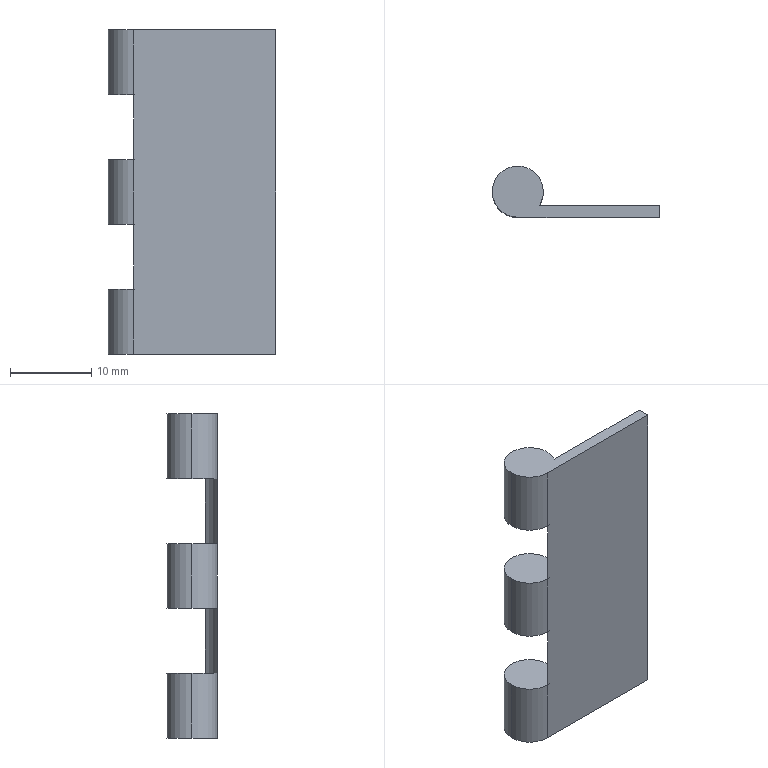Part | SolidWorks | features BaseBody 1 | 1 solid | 20 faces | box 20.65 x 6.3 x 40 mm | volume 1684 mm3 | cylinder 11 | plane 9 | commonest cylinder face diameters 6.3 x11
STEP:
#1=CARTESIAN_POINT('',(3.15,3.15,32.));
#2=VERTEX_POINT('',#1);
#3=CARTESIAN_POINT('',(-3.15,3.15,32.));
#4=VERTEX_POINT('',#3);
#5=CARTESIAN_POINT('',(0.,3.15,32.));
#6=DIRECTION('',(0.,0.,1.));
#7=DIRECTION('',(1.,0.,0.));
#8=AXIS2_PLACEMENT_3D('',#5,#6,#7);
#9=CIRCLE('',#8,3.15);
#10=EDGE_CURVE('',#2,#4,#9,.T.);
#11=ORIENTED_EDGE('',*,*,#10,.T.);
#12=CARTESIAN_POINT('',(-3.15,3.15,40.));
#13=VERTEX_POINT('',#12);
#14=CARTESIAN_POINT('',(-3.15,3.15,40.));
#15=DIRECTION('',(0.,0.,1.));
#16=VECTOR('',#15,1000.);
#17=LINE('',#14,#16);
#18=EDGE_CURVE('',#4,#13,#17,.T.);
#19=ORIENTED_EDGE('',*,*,#18,.T.);
#20=CARTESIAN_POINT('',(3.15,3.15,40.));
#21=VERTEX_POINT('',#20);
#22=CARTESIAN_POINT('',(0.,3.15,40.));
#23=DIRECTION('',(0.,0.,1.));
#24=DIRECTION('',(1.,0.,0.));
#25=AXIS2_PLACEMENT_3D('',#22,#23,#24);
#26=CIRCLE('',#25,3.15);
#27=EDGE_CURVE('',#21,#13,#26,.T.);
#28=ORIENTED_EDGE('',*,*,#27,.F.);
#29=CARTESIAN_POINT('',(3.15,3.15,40.));
#30=DIRECTION('',(0.,0.,1.));
#31=VECTOR('',#30,1000.);
#32=LINE('',#29,#31);
#33=EDGE_CURVE('',#2,#21,#32,.T.);
#34=ORIENTED_EDGE('',*,*,#33,.F.);
#35=EDGE_LOOP('',(#11,#19,#28,#34));
#36=FACE_OUTER_BOUND('',#35,.T.);
#37=CARTESIAN_POINT('',(0.,3.15,40.));
#38=DIRECTION('',(0.,0.,1.));
#39=DIRECTION('',(1.,0.,0.));
#40=AXIS2_PLACEMENT_3D('',#37,#38,#39);
#41=CYLINDRICAL_SURFACE('',#40,3.15);
#42=ADVANCED_FACE('',(#36),#41,.T.);
#43=CARTESIAN_POINT('',(2.683,1.5,32.));
#44=VERTEX_POINT('',#43);
#45=CARTESIAN_POINT('',(0.,3.15,32.));
#46=DIRECTION('',(0.,0.,1.));
#47=DIRECTION('',(1.,0.,0.));
#48=AXIS2_PLACEMENT_3D('',#45,#46,#47);
#49=CIRCLE('',#48,3.15);
#50=EDGE_CURVE('',#44,#2,#49,.T.);
#51=ORIENTED_EDGE('',*,*,#50,.T.);
#52=ORIENTED_EDGE('',*,*,#33,.T.);
#53=CARTESIAN_POINT('',(2.683,1.5,40.));
#54=VERTEX_POINT('',#53);
#55=CARTESIAN_POINT('',(0.,3.15,40.));
#56=DIRECTION('',(0.,0.,1.));
#57=DIRECTION('',(1.,0.,0.));
#58=AXIS2_PLACEMENT_3D('',#55,#56,#57);
#59=CIRCLE('',#58,3.15);
#60=EDGE_CURVE('',#54,#21,#59,.T.);
#61=ORIENTED_EDGE('',*,*,#60,.F.);
#62=CARTESIAN_POINT('',(2.683,1.5,40.));
#63=DIRECTION('',(0.,0.,-1.));
#64=VECTOR('',#63,1000.);
#65=LINE('',#62,#64);
#66=EDGE_CURVE('',#54,#44,#65,.T.);
#67=ORIENTED_EDGE('',*,*,#66,.T.);
#68=EDGE_LOOP('',(#51,#52,#61,#67));
#69=FACE_OUTER_BOUND('',#68,.T.);
#70=CARTESIAN_POINT('',(0.,3.15,40.));
#71=DIRECTION('',(0.,0.,1.));
#72=DIRECTION('',(1.,0.,0.));
#73=AXIS2_PLACEMENT_3D('',#70,#71,#72);
#74=CYLINDRICAL_SURFACE('',#73,3.15);
#75=ADVANCED_FACE('',(#69),#74,.T.);
#76=CARTESIAN_POINT('',(3.15,3.15,16.));
#77=VERTEX_POINT('',#76);
#78=CARTESIAN_POINT('',(-3.15,3.15,16.));
#79=VERTEX_POINT('',#78);
#80=CARTESIAN_POINT('',(0.,3.15,16.));
#81=DIRECTION('',(0.,0.,1.));
#82=DIRECTION('',(1.,0.,0.));
#83=AXIS2_PLACEMENT_3D('',#80,#81,#82);
#84=CIRCLE('',#83,3.15);
#85=EDGE_CURVE('',#77,#79,#84,.T.);
#86=ORIENTED_EDGE('',*,*,#85,.T.);
#87=CARTESIAN_POINT('',(-3.15,3.15,24.));
#88=VERTEX_POINT('',#87);
#89=CARTESIAN_POINT('',(-3.15,3.15,40.));
#90=DIRECTION('',(0.,0.,1.));
#91=VECTOR('',#90,1000.);
#92=LINE('',#89,#91);
#93=EDGE_CURVE('',#79,#88,#92,.T.);
#94=ORIENTED_EDGE('',*,*,#93,.T.);
#95=CARTESIAN_POINT('',(3.15,3.15,24.));
#96=VERTEX_POINT('',#95);
#97=CARTESIAN_POINT('',(0.,3.15,24.));
#98=DIRECTION('',(0.,0.,-1.));
#99=DIRECTION('',(1.,0.,0.));
#100=AXIS2_PLACEMENT_3D('',#97,#98,#99);
#101=CIRCLE('',#100,3.15);
#102=EDGE_CURVE('',#88,#96,#101,.T.);
#103=ORIENTED_EDGE('',*,*,#102,.T.);
#104=CARTESIAN_POINT('',(3.15,3.15,40.));
#105=DIRECTION('',(0.,0.,1.));
#106=VECTOR('',#105,1000.);
#107=LINE('',#104,#106);
#108=EDGE_CURVE('',#77,#96,#107,.T.);
#109=ORIENTED_EDGE('',*,*,#108,.F.);
#110=EDGE_LOOP('',(#86,#94,#103,#109));
#111=FACE_OUTER_BOUND('',#110,.T.);
#112=CARTESIAN_POINT('',(0.,3.15,40.));
#113=DIRECTION('',(0.,0.,1.));
#114=DIRECTION('',(1.,0.,0.));
#115=AXIS2_PLACEMENT_3D('',#112,#113,#114);
#116=CYLINDRICAL_SURFACE('',#115,3.15);
#117=ADVANCED_FACE('',(#111),#116,.T.);
#118=CARTESIAN_POINT('',(2.683,1.5,16.));
#119=VERTEX_POINT('',#118);
#120=CARTESIAN_POINT('',(0.,3.15,16.));
#121=DIRECTION('',(0.,0.,1.));
#122=DIRECTION('',(1.,0.,0.));
#123=AXIS2_PLACEMENT_3D('',#120,#121,#122);
#124=CIRCLE('',#123,3.15);
#125=EDGE_CURVE('',#119,#77,#124,.T.);
#126=ORIENTED_EDGE('',*,*,#125,.T.);
#127=ORIENTED_EDGE('',*,*,#108,.T.);
#128=CARTESIAN_POINT('',(2.683,1.5,24.));
#129=VERTEX_POINT('',#128);
#130=CARTESIAN_POINT('',(0.,3.15,24.));
#131=DIRECTION('',(0.,0.,-1.));
#132=DIRECTION('',(1.,0.,0.));
#133=AXIS2_PLACEMENT_3D('',#130,#131,#132);
#134=CIRCLE('',#133,3.15);
#135=EDGE_CURVE('',#96,#129,#134,.T.);
#136=ORIENTED_EDGE('',*,*,#135,.T.);
#137=CARTESIAN_POINT('',(2.683,1.5,40.));
#138=DIRECTION('',(0.,0.,-1.));
#139=VECTOR('',#138,1000.);
#140=LINE('',#137,#139);
#141=EDGE_CURVE('',#129,#119,#140,.T.);
#142=ORIENTED_EDGE('',*,*,#141,.T.);
#143=EDGE_LOOP('',(#126,#127,#136,#142));
#144=FACE_OUTER_BOUND('',#143,.T.);
#145=CARTESIAN_POINT('',(0.,3.15,40.));
#146=DIRECTION('',(0.,0.,1.));
#147=DIRECTION('',(1.,0.,0.));
#148=AXIS2_PLACEMENT_3D('',#145,#146,#147);
#149=CYLINDRICAL_SURFACE('',#148,3.15);
#150=ADVANCED_FACE('',(#144),#149,.T.);
#151=CARTESIAN_POINT('',(3.15,3.15,0.));
#152=VERTEX_POINT('',#151);
#153=CARTESIAN_POINT('',(-3.15,3.15,0.));
#154=VERTEX_POINT('',#153);
#155=CARTESIAN_POINT('',(0.,3.15,0.));
#156=DIRECTION('',(0.,0.,1.));
#157=DIRECTION('',(1.,0.,0.));
#158=AXIS2_PLACEMENT_3D('',#155,#156,#157);
#159=CIRCLE('',#158,3.15);
#160=EDGE_CURVE('',#152,#154,#159,.T.);
#161=ORIENTED_EDGE('',*,*,#160,.T.);
#162=CARTESIAN_POINT('',(-3.15,3.15,8.));
#163=VERTEX_POINT('',#162);
#164=CARTESIAN_POINT('',(-3.15,3.15,40.));
#165=DIRECTION('',(0.,0.,1.));
#166=VECTOR('',#165,1000.);
#167=LINE('',#164,#166);
#168=EDGE_CURVE('',#154,#163,#167,.T.);
#169=ORIENTED_EDGE('',*,*,#168,.T.);
#170=CARTESIAN_POINT('',(3.15,3.15,8.));
#171=VERTEX_POINT('',#170);
#172=CARTESIAN_POINT('',(0.,3.15,8.));
#173=DIRECTION('',(0.,0.,-1.));
#174=DIRECTION('',(1.,0.,0.));
#175=AXIS2_PLACEMENT_3D('',#172,#173,#174);
#176=CIRCLE('',#175,3.15);
#177=EDGE_CURVE('',#163,#171,#176,.T.);
#178=ORIENTED_EDGE('',*,*,#177,.T.);
#179=CARTESIAN_POINT('',(3.15,3.15,40.));
#180=DIRECTION('',(0.,0.,1.));
#181=VECTOR('',#180,1000.);
#182=LINE('',#179,#181);
#183=EDGE_CURVE('',#152,#171,#182,.T.);
#184=ORIENTED_EDGE('',*,*,#183,.F.);
#185=EDGE_LOOP('',(#161,#169,#178,#184));
#186=FACE_OUTER_BOUND('',#185,.T.);
#187=CARTESIAN_POINT('',(0.,3.15,40.));
#188=DIRECTION('',(0.,0.,1.));
#189=DIRECTION('',(1.,0.,0.));
#190=AXIS2_PLACEMENT_3D('',#187,#188,#189);
#191=CYLINDRICAL_SURFACE('',#190,3.15);
#192=ADVANCED_FACE('',(#186),#191,.T.);
#193=CARTESIAN_POINT('',(2.683,1.5,0.));
#194=VERTEX_POINT('',#193);
#195=CARTESIAN_POINT('',(0.,3.15,0.));
#196=DIRECTION('',(0.,0.,1.));
#197=DIRECTION('',(1.,0.,0.));
#198=AXIS2_PLACEMENT_3D('',#195,#196,#197);
#199=CIRCLE('',#198,3.15);
#200=EDGE_CURVE('',#194,#152,#199,.T.);
#201=ORIENTED_EDGE('',*,*,#200,.T.);
#202=ORIENTED_EDGE('',*,*,#183,.T.);
#203=CARTESIAN_POINT('',(2.683,1.5,8.));
#204=VERTEX_POINT('',#203);
#205=CARTESIAN_POINT('',(0.,3.15,8.));
#206=DIRECTION('',(0.,0.,-1.));
#207=DIRECTION('',(1.,0.,0.));
#208=AXIS2_PLACEMENT_3D('',#205,#206,#207);
#209=CIRCLE('',#208,3.15);
#210=EDGE_CURVE('',#171,#204,#209,.T.);
#211=ORIENTED_EDGE('',*,*,#210,.T.);
#212=CARTESIAN_POINT('',(2.683,1.5,40.));
#213=DIRECTION('',(0.,0.,-1.));
#214=VECTOR('',#213,1000.);
#215=LINE('',#212,#214);
#216=EDGE_CURVE('',#204,#194,#215,.T.);
#217=ORIENTED_EDGE('',*,*,#216,.T.);
#218=EDGE_LOOP('',(#201,#202,#211,#217));
#219=FACE_OUTER_BOUND('',#218,.T.);
#220=CARTESIAN_POINT('',(0.,3.15,40.));
#221=DIRECTION('',(0.,0.,1.));
#222=DIRECTION('',(1.,0.,0.));
#223=AXIS2_PLACEMENT_3D('',#220,#221,#222);
#224=CYLINDRICAL_SURFACE('',#223,3.15);
#225=ADVANCED_FACE('',(#219),#224,.T.);
#226=CARTESIAN_POINT('',(17.5,0.,40.));
#227=VERTEX_POINT('',#226);
#228=CARTESIAN_POINT('',(17.5,0.,0.));
#229=VERTEX_POINT('',#228);
#230=CARTESIAN_POINT('',(17.5,0.,40.));
#231=DIRECTION('',(0.,0.,-1.));
#232=VECTOR('',#231,1000.);
#233=LINE('',#230,#232);
#234=EDGE_CURVE('',#227,#229,#233,.T.);
#235=ORIENTED_EDGE('',*,*,#234,.F.);
#236=CARTESIAN_POINT('',(0.,0.,40.));
#237=VERTEX_POINT('',#236);
#238=CARTESIAN_POINT('',(0.,0.,40.));
#239=DIRECTION('',(1.,0.,0.));
#240=VECTOR('',#239,1000.);
#241=LINE('',#238,#240);
#242=EDGE_CURVE('',#237,#227,#241,.T.);
#243=ORIENTED_EDGE('',*,*,#242,.F.);
#244=CARTESIAN_POINT('',(0.,0.,32.));
#245=VERTEX_POINT('',#244);
#246=CARTESIAN_POINT('',(0.,0.,40.));
#247=DIRECTION('',(0.,0.,1.));
#248=VECTOR('',#247,1000.);
#249=LINE('',#246,#248);
#250=EDGE_CURVE('',#245,#237,#249,.T.);
#251=ORIENTED_EDGE('',*,*,#250,.F.);
#252=CARTESIAN_POINT('',(0.,0.,24.));
#253=VERTEX_POINT('',#252);
#254=CARTESIAN_POINT('',(0.,0.,40.));
#255=DIRECTION('',(0.,0.,1.));
#256=VECTOR('',#255,1000.);
#257=LINE('',#254,#256);
#258=EDGE_CURVE('',#253,#245,#257,.T.);
#259=ORIENTED_EDGE('',*,*,#258,.F.);
#260=CARTESIAN_POINT('',(0.,0.,16.));
#261=VERTEX_POINT('',#260);
#262=CARTESIAN_POINT('',(0.,0.,40.));
#263=DIRECTION('',(0.,0.,1.));
#264=VECTOR('',#263,1000.);
#265=LINE('',#262,#264);
#266=EDGE_CURVE('',#261,#253,#265,.T.);
#267=ORIENTED_EDGE('',*,*,#266,.F.);
#268=CARTESIAN_POINT('',(0.,0.,8.));
#269=VERTEX_POINT('',#268);
#270=CARTESIAN_POINT('',(0.,0.,40.));
#271=DIRECTION('',(0.,0.,1.));
#272=VECTOR('',#271,1000.);
#273=LINE('',#270,#272);
#274=EDGE_CURVE('',#269,#261,#273,.T.);
#275=ORIENTED_EDGE('',*,*,#274,.F.);
#276=CARTESIAN_POINT('',(0.,0.,0.));
#277=VERTEX_POINT('',#276);
#278=CARTESIAN_POINT('',(0.,0.,40.));
#279=DIRECTION('',(0.,0.,1.));
#280=VECTOR('',#279,1000.);
#281=LINE('',#278,#280);
#282=EDGE_CURVE('',#277,#269,#281,.T.);
#283=ORIENTED_EDGE('',*,*,#282,.F.);
#284=CARTESIAN_POINT('',(0.,0.,0.));
#285=DIRECTION('',(-1.,0.,0.));
#286=VECTOR('',#285,1000.);
#287=LINE('',#284,#286);
#288=EDGE_CURVE('',#229,#277,#287,.T.);
#289=ORIENTED_EDGE('',*,*,#288,.F.);
#290=EDGE_LOOP('',(#235,#243,#251,#259,#267,#275,#283,#289));
#291=FACE_OUTER_BOUND('',#290,.T.);
#292=CARTESIAN_POINT('',(0.,0.,40.));
#293=DIRECTION('',(0.,1.,0.));
#294=DIRECTION('',(0.,0.,1.));
#295=AXIS2_PLACEMENT_3D('',#292,#293,#294);
#296=PLANE('',#295);
#297=ADVANCED_FACE('',(#291),#296,.F.);
#298=CARTESIAN_POINT('',(17.5,1.5,0.));
#299=VERTEX_POINT('',#298);
#300=CARTESIAN_POINT('',(17.5,3.15,0.));
#301=DIRECTION('',(0.,1.,0.));
#302=VECTOR('',#301,1000.);
#303=LINE('',#300,#302);
#304=EDGE_CURVE('',#229,#299,#303,.T.);
#305=ORIENTED_EDGE('',*,*,#304,.F.);
#306=ORIENTED_EDGE('',*,*,#288,.T.);
#307=CARTESIAN_POINT('',(0.,3.15,0.));
#308=DIRECTION('',(0.,0.,1.));
#309=DIRECTION('',(1.,0.,0.));
#310=AXIS2_PLACEMENT_3D('',#307,#308,#309);
#311=CIRCLE('',#310,3.15);
#312=EDGE_CURVE('',#154,#277,#311,.T.);
#313=ORIENTED_EDGE('',*,*,#312,.F.);
#314=ORIENTED_EDGE('',*,*,#160,.F.);
#315=ORIENTED_EDGE('',*,*,#200,.F.);
#316=CARTESIAN_POINT('',(0.,1.5,0.));
#317=DIRECTION('',(-1.,0.,0.));
#318=VECTOR('',#317,1000.);
#319=LINE('',#316,#318);
#320=EDGE_CURVE('',#299,#194,#319,.T.);
#321=ORIENTED_EDGE('',*,*,#320,.F.);
#322=EDGE_LOOP('',(#305,#306,#313,#314,#315,#321));
#323=FACE_OUTER_BOUND('',#322,.T.);
#324=CARTESIAN_POINT('',(0.,3.15,0.));
#325=DIRECTION('',(0.,0.,1.));
#326=DIRECTION('',(1.,0.,0.));
#327=AXIS2_PLACEMENT_3D('',#324,#325,#326);
#328=PLANE('',#327);
#329=ADVANCED_FACE('',(#323),#328,.F.);
#330=CARTESIAN_POINT('',(17.5,1.5,40.));
#331=VERTEX_POINT('',#330);
#332=CARTESIAN_POINT('',(17.5,1.5,40.));
#333=DIRECTION('',(0.,0.,-1.));
#334=VECTOR('',#333,1000.);
#335=LINE('',#332,#334);
#336=EDGE_CURVE('',#331,#299,#335,.T.);
#337=ORIENTED_EDGE('',*,*,#336,.F.);
#338=CARTESIAN_POINT('',(17.5,0.,40.));
#339=DIRECTION('',(0.,1.,0.));
#340=VECTOR('',#339,1000.);
#341=LINE('',#338,#340);
#342=EDGE_CURVE('',#227,#331,#341,.T.);
#343=ORIENTED_EDGE('',*,*,#342,.F.);
#344=ORIENTED_EDGE('',*,*,#234,.T.);
#345=ORIENTED_EDGE('',*,*,#304,.T.);
#346=EDGE_LOOP('',(#337,#343,#344,#345));
#347=FACE_OUTER_BOUND('',#346,.T.);
#348=CARTESIAN_POINT('',(17.5,0.,40.));
#349=DIRECTION('',(-1.,0.,0.));
#350=DIRECTION('',(0.,0.,1.));
#351=AXIS2_PLACEMENT_3D('',#348,#349,#350);
#352=PLANE('',#351);
#353=ADVANCED_FACE('',(#347),#352,.F.);
#354=ORIENTED_EDGE('',*,*,#242,.T.);
#355=ORIENTED_EDGE('',*,*,#342,.T.);
#356=CARTESIAN_POINT('',(0.,1.5,40.));
#357=DIRECTION('',(-1.,0.,0.));
#358=VECTOR('',#357,1000.);
#359=LINE('',#356,#358);
#360=EDGE_CURVE('',#331,#54,#359,.T.);
#361=ORIENTED_EDGE('',*,*,#360,.T.);
#362=ORIENTED_EDGE('',*,*,#60,.T.);
#363=ORIENTED_EDGE('',*,*,#27,.T.);
#364=CARTESIAN_POINT('',(0.,3.15,40.));
#365=DIRECTION('',(0.,0.,1.));
#366=DIRECTION('',(1.,0.,0.));
#367=AXIS2_PLACEMENT_3D('',#364,#365,#366);
#368=CIRCLE('',#367,3.15);
#369=EDGE_CURVE('',#13,#237,#368,.T.);
#370=ORIENTED_EDGE('',*,*,#369,.T.);
#371=EDGE_LOOP('',(#354,#355,#361,#362,#363,#370));
#372=FACE_OUTER_BOUND('',#371,.T.);
#373=CARTESIAN_POINT('',(0.,3.15,40.));
#374=DIRECTION('',(0.,0.,1.));
#375=DIRECTION('',(1.,0.,0.));
#376=AXIS2_PLACEMENT_3D('',#373,#374,#375);
#377=PLANE('',#376);
#378=ADVANCED_FACE('',(#372),#377,.T.);
#379=ORIENTED_EDGE('',*,*,#18,.F.);
#380=CARTESIAN_POINT('',(0.,3.15,32.));
#381=DIRECTION('',(0.,0.,1.));
#382=DIRECTION('',(1.,0.,0.));
#383=AXIS2_PLACEMENT_3D('',#380,#381,#382);
#384=CIRCLE('',#383,3.15);
#385=EDGE_CURVE('',#4,#245,#384,.T.);
#386=ORIENTED_EDGE('',*,*,#385,.T.);
#387=ORIENTED_EDGE('',*,*,#250,.T.);
#388=ORIENTED_EDGE('',*,*,#369,.F.);
#389=EDGE_LOOP('',(#379,#386,#387,#388));
#390=FACE_OUTER_BOUND('',#389,.T.);
#391=CARTESIAN_POINT('',(0.,3.15,40.));
#392=DIRECTION('',(0.,0.,1.));
#393=DIRECTION('',(1.,0.,0.));
#394=AXIS2_PLACEMENT_3D('',#391,#392,#393);
#395=CYLINDRICAL_SURFACE('',#394,3.15);
#396=ADVANCED_FACE('',(#390),#395,.T.);
#397=CARTESIAN_POINT('',(0.,3.15,24.));
#398=DIRECTION('',(0.,0.,1.));
#399=DIRECTION('',(1.,0.,0.));
#400=AXIS2_PLACEMENT_3D('',#397,#398,#399);
#401=CIRCLE('',#400,3.15);
#402=EDGE_CURVE('',#253,#129,#401,.T.);
#403=ORIENTED_EDGE('',*,*,#402,.F.);
#404=ORIENTED_EDGE('',*,*,#258,.T.);
#405=CARTESIAN_POINT('',(0.,3.15,32.));
#406=DIRECTION('',(0.,0.,-1.));
#407=DIRECTION('',(1.,0.,0.));
#408=AXIS2_PLACEMENT_3D('',#405,#406,#407);
#409=CIRCLE('',#408,3.15);
#410=EDGE_CURVE('',#44,#245,#409,.T.);
#411=ORIENTED_EDGE('',*,*,#410,.F.);
#412=CARTESIAN_POINT('',(2.683,1.5,32.));
#413=DIRECTION('',(0.,0.,1.));
#414=VECTOR('',#413,1000.);
#415=LINE('',#412,#414);
#416=EDGE_CURVE('',#129,#44,#415,.T.);
#417=ORIENTED_EDGE('',*,*,#416,.F.);
#418=EDGE_LOOP('',(#403,#404,#411,#417));
#419=FACE_OUTER_BOUND('',#418,.T.);
#420=CARTESIAN_POINT('',(0.,3.15,32.));
#421=DIRECTION('',(0.,0.,1.));
#422=DIRECTION('',(1.,0.,0.));
#423=AXIS2_PLACEMENT_3D('',#420,#421,#422);
#424=CYLINDRICAL_SURFACE('',#423,3.15);
#425=ADVANCED_FACE('',(#419),#424,.F.);
#426=ORIENTED_EDGE('',*,*,#93,.F.);
#427=CARTESIAN_POINT('',(0.,3.15,16.));
#428=DIRECTION('',(0.,0.,1.));
#429=DIRECTION('',(1.,0.,0.));
#430=AXIS2_PLACEMENT_3D('',#427,#428,#429);
#431=CIRCLE('',#430,3.15);
#432=EDGE_CURVE('',#79,#261,#431,.T.);
#433=ORIENTED_EDGE('',*,*,#432,.T.);
#434=ORIENTED_EDGE('',*,*,#266,.T.);
#435=CARTESIAN_POINT('',(0.,3.15,24.));
#436=DIRECTION('',(0.,0.,-1.));
#437=DIRECTION('',(1.,0.,0.));
#438=AXIS2_PLACEMENT_3D('',#435,#436,#437);
#439=CIRCLE('',#438,3.15);
#440=EDGE_CURVE('',#253,#88,#439,.T.);
#441=ORIENTED_EDGE('',*,*,#440,.T.);
#442=EDGE_LOOP('',(#426,#433,#434,#441));
#443=FACE_OUTER_BOUND('',#442,.T.);
#444=CARTESIAN_POINT('',(0.,3.15,40.));
#445=DIRECTION('',(0.,0.,1.));
#446=DIRECTION('',(1.,0.,0.));
#447=AXIS2_PLACEMENT_3D('',#444,#445,#446);
#448=CYLINDRICAL_SURFACE('',#447,3.15);
#449=ADVANCED_FACE('',(#443),#448,.T.);
#450=CARTESIAN_POINT('',(0.,3.15,8.));
#451=DIRECTION('',(0.,0.,1.));
#452=DIRECTION('',(1.,0.,0.));
#453=AXIS2_PLACEMENT_3D('',#450,#451,#452);
#454=CIRCLE('',#453,3.15);
#455=EDGE_CURVE('',#269,#204,#454,.T.);
#456=ORIENTED_EDGE('',*,*,#455,.F.);
#457=ORIENTED_EDGE('',*,*,#274,.T.);
#458=CARTESIAN_POINT('',(0.,3.15,16.));
#459=DIRECTION('',(0.,0.,-1.));
#460=DIRECTION('',(1.,0.,0.));
#461=AXIS2_PLACEMENT_3D('',#458,#459,#460);
#462=CIRCLE('',#461,3.15);
#463=EDGE_CURVE('',#119,#261,#462,.T.);
#464=ORIENTED_EDGE('',*,*,#463,.F.);
#465=CARTESIAN_POINT('',(2.683,1.5,16.));
#466=DIRECTION('',(0.,0.,1.));
#467=VECTOR('',#466,1000.);
#468=LINE('',#465,#467);
#469=EDGE_CURVE('',#204,#119,#468,.T.);
#470=ORIENTED_EDGE('',*,*,#469,.F.);
#471=EDGE_LOOP('',(#456,#457,#464,#470));
#472=FACE_OUTER_BOUND('',#471,.T.);
#473=CARTESIAN_POINT('',(0.,3.15,16.));
#474=DIRECTION('',(0.,0.,1.));
#475=DIRECTION('',(1.,0.,0.));
#476=AXIS2_PLACEMENT_3D('',#473,#474,#475);
#477=CYLINDRICAL_SURFACE('',#476,3.15);
#478=ADVANCED_FACE('',(#472),#477,.F.);
#479=ORIENTED_EDGE('',*,*,#168,.F.);
#480=ORIENTED_EDGE('',*,*,#312,.T.);
#481=ORIENTED_EDGE('',*,*,#282,.T.);
#482=CARTESIAN_POINT('',(0.,3.15,8.));
#483=DIRECTION('',(0.,0.,-1.));
#484=DIRECTION('',(1.,0.,0.));
#485=AXIS2_PLACEMENT_3D('',#482,#483,#484);
#486=CIRCLE('',#485,3.15);
#487=EDGE_CURVE('',#269,#163,#486,.T.);
#488=ORIENTED_EDGE('',*,*,#487,.T.);
#489=EDGE_LOOP('',(#479,#480,#481,#488));
#490=FACE_OUTER_BOUND('',#489,.T.);
#491=CARTESIAN_POINT('',(0.,3.15,40.));
#492=DIRECTION('',(0.,0.,1.));
#493=DIRECTION('',(1.,0.,0.));
#494=AXIS2_PLACEMENT_3D('',#491,#492,#493);
#495=CYLINDRICAL_SURFACE('',#494,3.15);
#496=ADVANCED_FACE('',(#490),#495,.T.);
#497=ORIENTED_EDGE('',*,*,#216,.F.);
#498=ORIENTED_EDGE('',*,*,#469,.T.);
#499=ORIENTED_EDGE('',*,*,#141,.F.);
#500=ORIENTED_EDGE('',*,*,#416,.T.);
#501=ORIENTED_EDGE('',*,*,#66,.F.);
#502=ORIENTED_EDGE('',*,*,#360,.F.);
#503=ORIENTED_EDGE('',*,*,#336,.T.);
#504=ORIENTED_EDGE('',*,*,#320,.T.);
#505=EDGE_LOOP('',(#497,#498,#499,#500,#501,#502,#503,#504));
#506=FACE_OUTER_BOUND('',#505,.T.);
#507=CARTESIAN_POINT('',(17.5,1.5,40.));
#508=DIRECTION('',(0.,-1.,0.));
#509=DIRECTION('',(0.,0.,-1.));
#510=AXIS2_PLACEMENT_3D('',#507,#508,#509);
#511=PLANE('',#510);
#512=ADVANCED_FACE('',(#506),#511,.F.);
#513=ORIENTED_EDGE('',*,*,#50,.F.);
#514=ORIENTED_EDGE('',*,*,#410,.T.);
#515=ORIENTED_EDGE('',*,*,#385,.F.);
#516=ORIENTED_EDGE('',*,*,#10,.F.);
#517=EDGE_LOOP('',(#513,#514,#515,#516));
#518=FACE_OUTER_BOUND('',#517,.T.);
#519=CARTESIAN_POINT('',(0.,3.15,32.));
#520=DIRECTION('',(0.,0.,1.));
#521=DIRECTION('',(1.,0.,0.));
#522=AXIS2_PLACEMENT_3D('',#519,#520,#521);
#523=PLANE('',#522);
#524=ADVANCED_FACE('',(#518),#523,.F.);
#525=ORIENTED_EDGE('',*,*,#402,.T.);
#526=ORIENTED_EDGE('',*,*,#135,.F.);
#527=ORIENTED_EDGE('',*,*,#102,.F.);
#528=ORIENTED_EDGE('',*,*,#440,.F.);
#529=EDGE_LOOP('',(#525,#526,#527,#528));
#530=FACE_OUTER_BOUND('',#529,.T.);
#531=CARTESIAN_POINT('',(0.,3.15,24.));
#532=DIRECTION('',(0.,0.,1.));
#533=DIRECTION('',(1.,0.,0.));
#534=AXIS2_PLACEMENT_3D('',#531,#532,#533);
#535=PLANE('',#534);
#536=ADVANCED_FACE('',(#530),#535,.T.);
#537=ORIENTED_EDGE('',*,*,#125,.F.);
#538=ORIENTED_EDGE('',*,*,#463,.T.);
#539=ORIENTED_EDGE('',*,*,#432,.F.);
#540=ORIENTED_EDGE('',*,*,#85,.F.);
#541=EDGE_LOOP('',(#537,#538,#539,#540));
#542=FACE_OUTER_BOUND('',#541,.T.);
#543=CARTESIAN_POINT('',(0.,3.15,16.));
#544=DIRECTION('',(0.,0.,1.));
#545=DIRECTION('',(1.,0.,0.));
#546=AXIS2_PLACEMENT_3D('',#543,#544,#545);
#547=PLANE('',#546);
#548=ADVANCED_FACE('',(#542),#547,.F.);
#549=ORIENTED_EDGE('',*,*,#455,.T.);
#550=ORIENTED_EDGE('',*,*,#210,.F.);
#551=ORIENTED_EDGE('',*,*,#177,.F.);
#552=ORIENTED_EDGE('',*,*,#487,.F.);
#553=EDGE_LOOP('',(#549,#550,#551,#552));
#554=FACE_OUTER_BOUND('',#553,.T.);
#555=CARTESIAN_POINT('',(0.,3.15,8.));
#556=DIRECTION('',(0.,0.,1.));
#557=DIRECTION('',(1.,0.,0.));
#558=AXIS2_PLACEMENT_3D('',#555,#556,#557);
#559=PLANE('',#558);
#560=ADVANCED_FACE('',(#554),#559,.T.);
#561=CLOSED_SHELL('',(#42,#75,#117,#150,#192,#225,#297,#329,#353,#378,#396,#425,#449,#478,#496,#512,#524,#536,#548,#560));
#562=MANIFOLD_SOLID_BREP('',#561);
#563=CARTESIAN_POINT('',(0.,0.,0.));
#564=DIRECTION('',(0.,0.,1.));
#565=DIRECTION('',(1.,0.,0.));
#566=AXIS2_PLACEMENT_3D('',#563,#564,#565);
#567=(LENGTH_UNIT()NAMED_UNIT(*)SI_UNIT(.MILLI.,.METRE.));
#568=UNCERTAINTY_MEASURE_WITH_UNIT(LENGTH_MEASURE(0.00001),#567,'','');
#569=(NAMED_UNIT(*)PLANE_ANGLE_UNIT()SI_UNIT($,.RADIAN.));
#570=(NAMED_UNIT(*)SI_UNIT($,.STERADIAN.)SOLID_ANGLE_UNIT());
#571=(GEOMETRIC_REPRESENTATION_CONTEXT(3)GLOBAL_UNCERTAINTY_ASSIGNED_CONTEXT((#568))GLOBAL_UNIT_ASSIGNED_CONTEXT((#567,#569,#570))REPRESENTATION_CONTEXT('',''));
#572=ADVANCED_BREP_SHAPE_REPRESENTATION('',(#562,#566),#571);